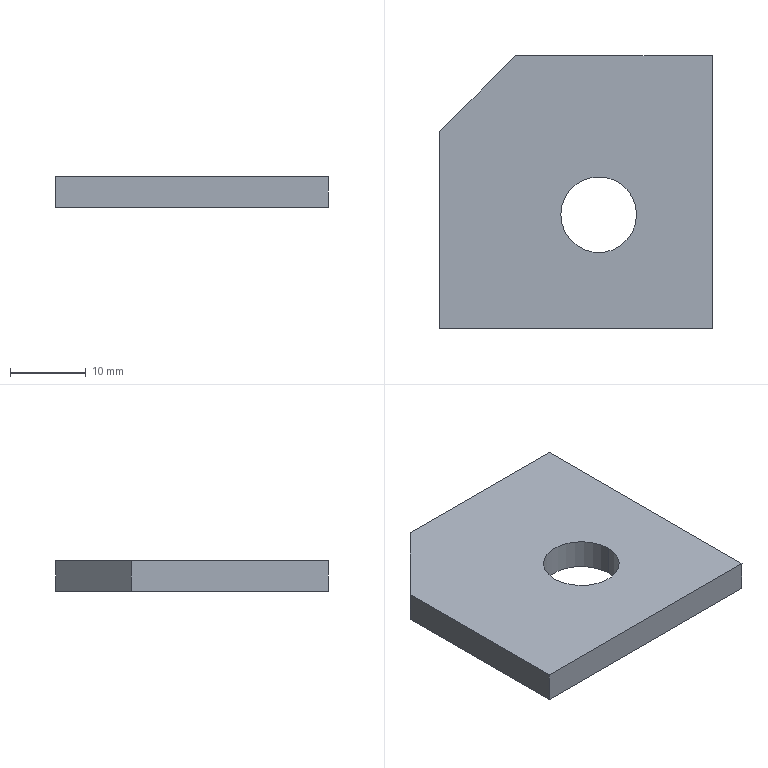Part | SolidWorks | features Chamfer 1, Extrusion 1, HoleWzd 1 | 1 solid | 9 faces | box 36 x 36 x 4 mm | volume 4670 mm3 | plane 7 | cylinder 2 | commonest cylinder face diameters 10 x2
STEP:
#1=CARTESIAN_POINT('',(16.,15.,0.));
#2=VERTEX_POINT('',#1);
#3=CARTESIAN_POINT('',(26.,15.,0.));
#4=VERTEX_POINT('',#3);
#5=CARTESIAN_POINT('',(21.,15.,0.));
#6=DIRECTION('',(0.,0.,1.));
#7=DIRECTION('',(1.,0.,0.));
#8=AXIS2_PLACEMENT_3D('',#5,#6,#7);
#9=CIRCLE('',#8,5.);
#10=EDGE_CURVE('',#2,#4,#9,.T.);
#11=ORIENTED_EDGE('',*,*,#10,.F.);
#12=CARTESIAN_POINT('',(16.,15.,4.));
#13=VERTEX_POINT('',#12);
#14=CARTESIAN_POINT('',(16.,15.,4.));
#15=DIRECTION('',(0.,0.,1.));
#16=VECTOR('',#15,1000.);
#17=LINE('',#14,#16);
#18=EDGE_CURVE('',#2,#13,#17,.T.);
#19=ORIENTED_EDGE('',*,*,#18,.T.);
#20=CARTESIAN_POINT('',(26.,15.,4.));
#21=VERTEX_POINT('',#20);
#22=CARTESIAN_POINT('',(21.,15.,4.));
#23=DIRECTION('',(0.,0.,1.));
#24=DIRECTION('',(1.,0.,0.));
#25=AXIS2_PLACEMENT_3D('',#22,#23,#24);
#26=CIRCLE('',#25,5.);
#27=EDGE_CURVE('',#13,#21,#26,.T.);
#28=ORIENTED_EDGE('',*,*,#27,.T.);
#29=CARTESIAN_POINT('',(26.,15.,4.));
#30=DIRECTION('',(0.,0.,1.));
#31=VECTOR('',#30,1000.);
#32=LINE('',#29,#31);
#33=EDGE_CURVE('',#4,#21,#32,.T.);
#34=ORIENTED_EDGE('',*,*,#33,.F.);
#35=EDGE_LOOP('',(#11,#19,#28,#34));
#36=FACE_OUTER_BOUND('',#35,.T.);
#37=CARTESIAN_POINT('',(21.,15.,4.));
#38=DIRECTION('',(0.,0.,1.));
#39=DIRECTION('',(1.,0.,0.));
#40=AXIS2_PLACEMENT_3D('',#37,#38,#39);
#41=CYLINDRICAL_SURFACE('',#40,5.);
#42=ADVANCED_FACE('',(#36),#41,.F.);
#43=CARTESIAN_POINT('',(0.,26.,4.));
#44=VERTEX_POINT('',#43);
#45=CARTESIAN_POINT('',(0.,0.,4.));
#46=VERTEX_POINT('',#45);
#47=CARTESIAN_POINT('',(0.,0.,4.));
#48=DIRECTION('',(0.,-1.,0.));
#49=VECTOR('',#48,1000.);
#50=LINE('',#47,#49);
#51=EDGE_CURVE('',#44,#46,#50,.T.);
#52=ORIENTED_EDGE('',*,*,#51,.F.);
#53=CARTESIAN_POINT('',(0.,26.,0.));
#54=VERTEX_POINT('',#53);
#55=CARTESIAN_POINT('',(0.,26.,4.));
#56=DIRECTION('',(0.,0.,-1.));
#57=VECTOR('',#56,1000.);
#58=LINE('',#55,#57);
#59=EDGE_CURVE('',#44,#54,#58,.T.);
#60=ORIENTED_EDGE('',*,*,#59,.T.);
#61=CARTESIAN_POINT('',(0.,0.,0.));
#62=VERTEX_POINT('',#61);
#63=CARTESIAN_POINT('',(0.,0.,0.));
#64=DIRECTION('',(0.,-1.,0.));
#65=VECTOR('',#64,1000.);
#66=LINE('',#63,#65);
#67=EDGE_CURVE('',#54,#62,#66,.T.);
#68=ORIENTED_EDGE('',*,*,#67,.T.);
#69=CARTESIAN_POINT('',(0.,0.,4.));
#70=DIRECTION('',(0.,0.,-1.));
#71=VECTOR('',#70,1000.);
#72=LINE('',#69,#71);
#73=EDGE_CURVE('',#46,#62,#72,.T.);
#74=ORIENTED_EDGE('',*,*,#73,.F.);
#75=EDGE_LOOP('',(#52,#60,#68,#74));
#76=FACE_OUTER_BOUND('',#75,.T.);
#77=CARTESIAN_POINT('',(0.,0.,4.));
#78=DIRECTION('',(1.,0.,0.));
#79=DIRECTION('',(0.,0.,-1.));
#80=AXIS2_PLACEMENT_3D('',#77,#78,#79);
#81=PLANE('',#80);
#82=ADVANCED_FACE('',(#76),#81,.F.);
#83=CARTESIAN_POINT('',(36.,0.,0.));
#84=VERTEX_POINT('',#83);
#85=CARTESIAN_POINT('',(0.,0.,0.));
#86=DIRECTION('',(1.,0.,0.));
#87=VECTOR('',#86,1000.);
#88=LINE('',#85,#87);
#89=EDGE_CURVE('',#62,#84,#88,.T.);
#90=ORIENTED_EDGE('',*,*,#89,.T.);
#91=CARTESIAN_POINT('',(36.,0.,4.));
#92=VERTEX_POINT('',#91);
#93=CARTESIAN_POINT('',(36.,0.,4.));
#94=DIRECTION('',(0.,0.,-1.));
#95=VECTOR('',#94,1000.);
#96=LINE('',#93,#95);
#97=EDGE_CURVE('',#92,#84,#96,.T.);
#98=ORIENTED_EDGE('',*,*,#97,.F.);
#99=CARTESIAN_POINT('',(0.,0.,4.));
#100=DIRECTION('',(1.,0.,0.));
#101=VECTOR('',#100,1000.);
#102=LINE('',#99,#101);
#103=EDGE_CURVE('',#46,#92,#102,.T.);
#104=ORIENTED_EDGE('',*,*,#103,.F.);
#105=ORIENTED_EDGE('',*,*,#73,.T.);
#106=EDGE_LOOP('',(#90,#98,#104,#105));
#107=FACE_OUTER_BOUND('',#106,.T.);
#108=CARTESIAN_POINT('',(0.,0.,4.));
#109=DIRECTION('',(0.,1.,0.));
#110=DIRECTION('',(0.,0.,1.));
#111=AXIS2_PLACEMENT_3D('',#108,#109,#110);
#112=PLANE('',#111);
#113=ADVANCED_FACE('',(#107),#112,.F.);
#114=CARTESIAN_POINT('',(36.,36.,0.));
#115=VERTEX_POINT('',#114);
#116=CARTESIAN_POINT('',(36.,0.,0.));
#117=DIRECTION('',(0.,1.,0.));
#118=VECTOR('',#117,1000.);
#119=LINE('',#116,#118);
#120=EDGE_CURVE('',#84,#115,#119,.T.);
#121=ORIENTED_EDGE('',*,*,#120,.T.);
#122=CARTESIAN_POINT('',(36.,36.,4.));
#123=VERTEX_POINT('',#122);
#124=CARTESIAN_POINT('',(36.,36.,4.));
#125=DIRECTION('',(0.,0.,-1.));
#126=VECTOR('',#125,1000.);
#127=LINE('',#124,#126);
#128=EDGE_CURVE('',#123,#115,#127,.T.);
#129=ORIENTED_EDGE('',*,*,#128,.F.);
#130=CARTESIAN_POINT('',(36.,0.,4.));
#131=DIRECTION('',(0.,1.,0.));
#132=VECTOR('',#131,1000.);
#133=LINE('',#130,#132);
#134=EDGE_CURVE('',#92,#123,#133,.T.);
#135=ORIENTED_EDGE('',*,*,#134,.F.);
#136=ORIENTED_EDGE('',*,*,#97,.T.);
#137=EDGE_LOOP('',(#121,#129,#135,#136));
#138=FACE_OUTER_BOUND('',#137,.T.);
#139=CARTESIAN_POINT('',(36.,0.,4.));
#140=DIRECTION('',(-1.,0.,0.));
#141=DIRECTION('',(0.,-1.,0.));
#142=AXIS2_PLACEMENT_3D('',#139,#140,#141);
#143=PLANE('',#142);
#144=ADVANCED_FACE('',(#138),#143,.F.);
#145=CARTESIAN_POINT('',(10.,36.,0.));
#146=VERTEX_POINT('',#145);
#147=CARTESIAN_POINT('',(0.,36.,0.));
#148=DIRECTION('',(-1.,0.,0.));
#149=VECTOR('',#148,1000.);
#150=LINE('',#147,#149);
#151=EDGE_CURVE('',#115,#146,#150,.T.);
#152=ORIENTED_EDGE('',*,*,#151,.T.);
#153=CARTESIAN_POINT('',(10.,36.,4.));
#154=VERTEX_POINT('',#153);
#155=CARTESIAN_POINT('',(10.,36.,4.));
#156=DIRECTION('',(0.,0.,1.));
#157=VECTOR('',#156,1000.);
#158=LINE('',#155,#157);
#159=EDGE_CURVE('',#146,#154,#158,.T.);
#160=ORIENTED_EDGE('',*,*,#159,.T.);
#161=CARTESIAN_POINT('',(0.,36.,4.));
#162=DIRECTION('',(-1.,0.,0.));
#163=VECTOR('',#162,1000.);
#164=LINE('',#161,#163);
#165=EDGE_CURVE('',#123,#154,#164,.T.);
#166=ORIENTED_EDGE('',*,*,#165,.F.);
#167=ORIENTED_EDGE('',*,*,#128,.T.);
#168=EDGE_LOOP('',(#152,#160,#166,#167));
#169=FACE_OUTER_BOUND('',#168,.T.);
#170=CARTESIAN_POINT('',(0.,36.,4.));
#171=DIRECTION('',(0.,-1.,0.));
#172=DIRECTION('',(0.,0.,-1.));
#173=AXIS2_PLACEMENT_3D('',#170,#171,#172);
#174=PLANE('',#173);
#175=ADVANCED_FACE('',(#169),#174,.F.);
#176=CARTESIAN_POINT('',(21.,15.,4.));
#177=DIRECTION('',(0.,0.,1.));
#178=DIRECTION('',(1.,0.,0.));
#179=AXIS2_PLACEMENT_3D('',#176,#177,#178);
#180=CIRCLE('',#179,5.);
#181=EDGE_CURVE('',#21,#13,#180,.T.);
#182=ORIENTED_EDGE('',*,*,#181,.F.);
#183=ORIENTED_EDGE('',*,*,#27,.F.);
#184=EDGE_LOOP('',(#182,#183));
#185=FACE_BOUND('',#184,.T.);
#186=ORIENTED_EDGE('',*,*,#165,.T.);
#187=CARTESIAN_POINT('',(0.,26.,4.));
#188=DIRECTION('',(-0.7071,-0.7071,0.));
#189=VECTOR('',#188,1000.);
#190=LINE('',#187,#189);
#191=EDGE_CURVE('',#154,#44,#190,.T.);
#192=ORIENTED_EDGE('',*,*,#191,.T.);
#193=ORIENTED_EDGE('',*,*,#51,.T.);
#194=ORIENTED_EDGE('',*,*,#103,.T.);
#195=ORIENTED_EDGE('',*,*,#134,.T.);
#196=EDGE_LOOP('',(#186,#192,#193,#194,#195));
#197=FACE_OUTER_BOUND('',#196,.T.);
#198=CARTESIAN_POINT('',(0.,0.,4.));
#199=DIRECTION('',(0.,0.,-1.));
#200=DIRECTION('',(-1.,0.,0.));
#201=AXIS2_PLACEMENT_3D('',#198,#199,#200);
#202=PLANE('',#201);
#203=ADVANCED_FACE('',(#185,#197),#202,.F.);
#204=CARTESIAN_POINT('',(21.,15.,0.));
#205=DIRECTION('',(0.,0.,1.));
#206=DIRECTION('',(1.,0.,0.));
#207=AXIS2_PLACEMENT_3D('',#204,#205,#206);
#208=CIRCLE('',#207,5.);
#209=EDGE_CURVE('',#4,#2,#208,.T.);
#210=ORIENTED_EDGE('',*,*,#209,.T.);
#211=ORIENTED_EDGE('',*,*,#10,.T.);
#212=EDGE_LOOP('',(#210,#211));
#213=FACE_BOUND('',#212,.T.);
#214=ORIENTED_EDGE('',*,*,#67,.F.);
#215=CARTESIAN_POINT('',(-13.,13.,0.));
#216=DIRECTION('',(0.7071,0.7071,0.));
#217=VECTOR('',#216,1000.);
#218=LINE('',#215,#217);
#219=EDGE_CURVE('',#54,#146,#218,.T.);
#220=ORIENTED_EDGE('',*,*,#219,.T.);
#221=ORIENTED_EDGE('',*,*,#151,.F.);
#222=ORIENTED_EDGE('',*,*,#120,.F.);
#223=ORIENTED_EDGE('',*,*,#89,.F.);
#224=EDGE_LOOP('',(#214,#220,#221,#222,#223));
#225=FACE_OUTER_BOUND('',#224,.T.);
#226=CARTESIAN_POINT('',(0.,0.,0.));
#227=DIRECTION('',(0.,0.,-1.));
#228=DIRECTION('',(-1.,0.,0.));
#229=AXIS2_PLACEMENT_3D('',#226,#227,#228);
#230=PLANE('',#229);
#231=ADVANCED_FACE('',(#213,#225),#230,.T.);
#232=ORIENTED_EDGE('',*,*,#191,.F.);
#233=ORIENTED_EDGE('',*,*,#159,.F.);
#234=ORIENTED_EDGE('',*,*,#219,.F.);
#235=ORIENTED_EDGE('',*,*,#59,.F.);
#236=EDGE_LOOP('',(#232,#233,#234,#235));
#237=FACE_OUTER_BOUND('',#236,.T.);
#238=CARTESIAN_POINT('',(0.,26.,4.));
#239=DIRECTION('',(0.7071,-0.7071,0.));
#240=DIRECTION('',(0.,0.,-1.));
#241=AXIS2_PLACEMENT_3D('',#238,#239,#240);
#242=PLANE('',#241);
#243=ADVANCED_FACE('',(#237),#242,.F.);
#244=ORIENTED_EDGE('',*,*,#18,.F.);
#245=ORIENTED_EDGE('',*,*,#209,.F.);
#246=ORIENTED_EDGE('',*,*,#33,.T.);
#247=ORIENTED_EDGE('',*,*,#181,.T.);
#248=EDGE_LOOP('',(#244,#245,#246,#247));
#249=FACE_OUTER_BOUND('',#248,.T.);
#250=CARTESIAN_POINT('',(21.,15.,4.));
#251=DIRECTION('',(0.,0.,1.));
#252=DIRECTION('',(1.,0.,0.));
#253=AXIS2_PLACEMENT_3D('',#250,#251,#252);
#254=CYLINDRICAL_SURFACE('',#253,5.);
#255=ADVANCED_FACE('',(#249),#254,.F.);
#256=CLOSED_SHELL('',(#42,#82,#113,#144,#175,#203,#231,#243,#255));
#257=MANIFOLD_SOLID_BREP('',#256);
#258=CARTESIAN_POINT('',(0.,0.,0.));
#259=DIRECTION('',(0.,0.,1.));
#260=DIRECTION('',(1.,0.,0.));
#261=AXIS2_PLACEMENT_3D('',#258,#259,#260);
#262=(LENGTH_UNIT()NAMED_UNIT(*)SI_UNIT(.MILLI.,.METRE.));
#263=UNCERTAINTY_MEASURE_WITH_UNIT(LENGTH_MEASURE(0.00001),#262,'','');
#264=(NAMED_UNIT(*)PLANE_ANGLE_UNIT()SI_UNIT($,.RADIAN.));
#265=(NAMED_UNIT(*)SI_UNIT($,.STERADIAN.)SOLID_ANGLE_UNIT());
#266=(GEOMETRIC_REPRESENTATION_CONTEXT(3)GLOBAL_UNCERTAINTY_ASSIGNED_CONTEXT((#263))GLOBAL_UNIT_ASSIGNED_CONTEXT((#262,#264,#265))REPRESENTATION_CONTEXT('',''));
#267=ADVANCED_BREP_SHAPE_REPRESENTATION('',(#257,#261),#266);